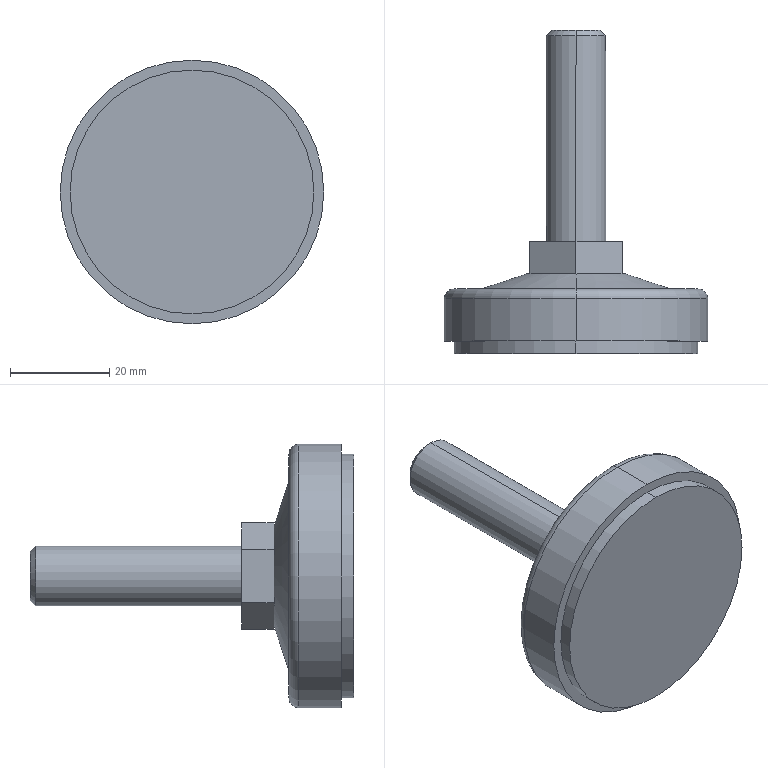Part | STEP file | JAJ-65_adjusters | 1 solid | 35 faces | box 53 x 65 x 53 mm | volume 36497 mm3 | plane 23 | cylinder 6 | cone 4 | torus 2 | commonest cylinder face diameters 12 x2 49 x2 53 x2
STEP:
#1=CARTESIAN_POINT('',(0.000000001,-1.074,6.));
#2=VERTEX_POINT('',#1);
#3=CARTESIAN_POINT('',(-0.000000001,-1.074,-6.));
#4=VERTEX_POINT('',#3);
#5=CARTESIAN_POINT('',(0.,-1.074,0.));
#6=DIRECTION('',(0.,-1.,0.));
#7=DIRECTION('',(0.,0.,-1.));
#8=AXIS2_PLACEMENT_3D('',#5,#6,#7);
#9=CIRCLE('',#8,6.);
#10=EDGE_CURVE('',#2,#4,#9,.T.);
#11=ORIENTED_EDGE('',*,*,#10,.T.);
#12=CARTESIAN_POINT('',(-0.000000005,-42.5,-6.));
#13=VERTEX_POINT('',#12);
#14=CARTESIAN_POINT('',(-0.000000005,-65.,-6.));
#15=DIRECTION('',(0.,-1.,0.));
#16=VECTOR('',#15,1000.);
#17=LINE('',#14,#16);
#18=EDGE_CURVE('',#4,#13,#17,.T.);
#19=ORIENTED_EDGE('',*,*,#18,.T.);
#20=CARTESIAN_POINT('',(-0.000000007,-42.5,6.));
#21=VERTEX_POINT('',#20);
#22=CARTESIAN_POINT('',(0.,-42.5,0.));
#23=DIRECTION('',(0.,1.,0.));
#24=DIRECTION('',(-0.000000001,0.,1.));
#25=AXIS2_PLACEMENT_3D('',#22,#23,#24);
#26=CIRCLE('',#25,6.);
#27=EDGE_CURVE('',#13,#21,#26,.T.);
#28=ORIENTED_EDGE('',*,*,#27,.T.);
#29=CARTESIAN_POINT('',(0.000000005,-65.,6.));
#30=DIRECTION('',(0.,-1.,0.));
#31=VECTOR('',#30,1000.);
#32=LINE('',#29,#31);
#33=EDGE_CURVE('',#2,#21,#32,.T.);
#34=ORIENTED_EDGE('',*,*,#33,.F.);
#35=EDGE_LOOP('',(#11,#19,#28,#34));
#36=FACE_OUTER_BOUND('',#35,.T.);
#37=CARTESIAN_POINT('',(0.,-65.,0.));
#38=DIRECTION('',(0.,-1.,0.));
#39=DIRECTION('',(0.000000001,0.,1.));
#40=AXIS2_PLACEMENT_3D('',#37,#38,#39);
#41=CYLINDRICAL_SURFACE('',#40,6.);
#42=ADVANCED_FACE('',(#36),#41,.T.);
#43=CARTESIAN_POINT('',(0.000000001,0.,4.927));
#44=VERTEX_POINT('',#43);
#45=CARTESIAN_POINT('',(-0.000000001,0.,-4.927));
#46=VERTEX_POINT('',#45);
#47=CARTESIAN_POINT('',(0.,0.,0.));
#48=DIRECTION('',(0.,-1.,0.));
#49=DIRECTION('',(0.,0.,-1.));
#50=AXIS2_PLACEMENT_3D('',#47,#48,#49);
#51=CIRCLE('',#50,4.927);
#52=EDGE_CURVE('',#44,#46,#51,.T.);
#53=ORIENTED_EDGE('',*,*,#52,.T.);
#54=CARTESIAN_POINT('',(-0.000000001,-1.074,-6.));
#55=DIRECTION('',(0.,-0.7071,-0.7071));
#56=VECTOR('',#55,1000.);
#57=LINE('',#54,#56);
#58=EDGE_CURVE('',#46,#4,#57,.T.);
#59=ORIENTED_EDGE('',*,*,#58,.T.);
#60=ORIENTED_EDGE('',*,*,#10,.F.);
#61=CARTESIAN_POINT('',(0.000000001,-1.074,6.));
#62=DIRECTION('',(0.,-0.7071,0.7071));
#63=VECTOR('',#62,1000.);
#64=LINE('',#61,#63);
#65=EDGE_CURVE('',#44,#2,#64,.T.);
#66=ORIENTED_EDGE('',*,*,#65,.F.);
#67=EDGE_LOOP('',(#53,#59,#60,#66));
#68=FACE_OUTER_BOUND('',#67,.T.);
#69=CARTESIAN_POINT('',(0.,-1.074,0.));
#70=DIRECTION('',(0.,-1.,0.));
#71=DIRECTION('',(0.,0.,1.));
#72=AXIS2_PLACEMENT_3D('',#69,#70,#71);
#73=CONICAL_SURFACE('',#72,6.,0.7854);
#74=ADVANCED_FACE('',(#68),#73,.T.);
#75=CARTESIAN_POINT('',(0.,-62.5,24.5));
#76=VERTEX_POINT('',#75);
#77=CARTESIAN_POINT('',(0.,-62.5,-24.5));
#78=VERTEX_POINT('',#77);
#79=CARTESIAN_POINT('',(0.,-62.5,0.));
#80=DIRECTION('',(0.,-1.,0.));
#81=DIRECTION('',(0.,0.,-1.));
#82=AXIS2_PLACEMENT_3D('',#79,#80,#81);
#83=CIRCLE('',#82,24.5);
#84=EDGE_CURVE('',#76,#78,#83,.T.);
#85=ORIENTED_EDGE('',*,*,#84,.T.);
#86=CARTESIAN_POINT('',(0.,-65.,-24.5));
#87=VERTEX_POINT('',#86);
#88=CARTESIAN_POINT('',(0.,-65.,-24.5));
#89=DIRECTION('',(0.,-1.,0.));
#90=VECTOR('',#89,1000.);
#91=LINE('',#88,#90);
#92=EDGE_CURVE('',#78,#87,#91,.T.);
#93=ORIENTED_EDGE('',*,*,#92,.T.);
#94=CARTESIAN_POINT('',(-0.000000029,-65.,24.5));
#95=VERTEX_POINT('',#94);
#96=CARTESIAN_POINT('',(0.,-65.,0.));
#97=DIRECTION('',(0.,-1.,0.));
#98=DIRECTION('',(-0.000000001,0.,1.));
#99=AXIS2_PLACEMENT_3D('',#96,#97,#98);
#100=CIRCLE('',#99,24.5);
#101=EDGE_CURVE('',#95,#87,#100,.T.);
#102=ORIENTED_EDGE('',*,*,#101,.F.);
#103=CARTESIAN_POINT('',(0.,-65.,24.5));
#104=DIRECTION('',(0.,-1.,0.));
#105=VECTOR('',#104,1000.);
#106=LINE('',#103,#105);
#107=EDGE_CURVE('',#76,#95,#106,.T.);
#108=ORIENTED_EDGE('',*,*,#107,.F.);
#109=EDGE_LOOP('',(#85,#93,#102,#108));
#110=FACE_OUTER_BOUND('',#109,.T.);
#111=CARTESIAN_POINT('',(0.,-65.,0.));
#112=DIRECTION('',(0.,-1.,0.));
#113=DIRECTION('',(0.,0.,1.));
#114=AXIS2_PLACEMENT_3D('',#111,#112,#113);
#115=CYLINDRICAL_SURFACE('',#114,24.5);
#116=ADVANCED_FACE('',(#110),#115,.T.);
#117=CARTESIAN_POINT('',(0.,-54.,26.5));
#118=VERTEX_POINT('',#117);
#119=CARTESIAN_POINT('',(0.,-54.,-26.5));
#120=VERTEX_POINT('',#119);
#121=CARTESIAN_POINT('',(0.,-54.,0.));
#122=DIRECTION('',(0.,-1.,0.));
#123=DIRECTION('',(0.,0.,-1.));
#124=AXIS2_PLACEMENT_3D('',#121,#122,#123);
#125=CIRCLE('',#124,26.5);
#126=EDGE_CURVE('',#118,#120,#125,.T.);
#127=ORIENTED_EDGE('',*,*,#126,.T.);
#128=CARTESIAN_POINT('',(0.,-62.5,-26.5));
#129=VERTEX_POINT('',#128);
#130=CARTESIAN_POINT('',(0.,-65.,-26.5));
#131=DIRECTION('',(0.,-1.,0.));
#132=VECTOR('',#131,1000.);
#133=LINE('',#130,#132);
#134=EDGE_CURVE('',#120,#129,#133,.T.);
#135=ORIENTED_EDGE('',*,*,#134,.T.);
#136=CARTESIAN_POINT('',(0.,-62.5,26.5));
#137=VERTEX_POINT('',#136);
#138=CARTESIAN_POINT('',(0.,-62.5,0.));
#139=DIRECTION('',(0.,-1.,0.));
#140=DIRECTION('',(0.,0.,1.));
#141=AXIS2_PLACEMENT_3D('',#138,#139,#140);
#142=CIRCLE('',#141,26.5);
#143=EDGE_CURVE('',#137,#129,#142,.T.);
#144=ORIENTED_EDGE('',*,*,#143,.F.);
#145=CARTESIAN_POINT('',(0.,-65.,26.5));
#146=DIRECTION('',(0.,-1.,0.));
#147=VECTOR('',#146,1000.);
#148=LINE('',#145,#147);
#149=EDGE_CURVE('',#118,#137,#148,.T.);
#150=ORIENTED_EDGE('',*,*,#149,.F.);
#151=EDGE_LOOP('',(#127,#135,#144,#150));
#152=FACE_OUTER_BOUND('',#151,.T.);
#153=CARTESIAN_POINT('',(0.,-65.,0.));
#154=DIRECTION('',(0.,-1.,0.));
#155=DIRECTION('',(0.,0.,1.));
#156=AXIS2_PLACEMENT_3D('',#153,#154,#155);
#157=CYLINDRICAL_SURFACE('',#156,26.5);
#158=ADVANCED_FACE('',(#152),#157,.T.);
#159=CARTESIAN_POINT('',(0.,-52.,24.5));
#160=VERTEX_POINT('',#159);
#161=CARTESIAN_POINT('',(0.,-52.,-24.5));
#162=VERTEX_POINT('',#161);
#163=CARTESIAN_POINT('',(0.,-52.,0.));
#164=DIRECTION('',(0.,-1.,0.));
#165=DIRECTION('',(0.,0.,-1.));
#166=AXIS2_PLACEMENT_3D('',#163,#164,#165);
#167=CIRCLE('',#166,24.5);
#168=EDGE_CURVE('',#160,#162,#167,.T.);
#169=ORIENTED_EDGE('',*,*,#168,.T.);
#170=CARTESIAN_POINT('',(0.,-54.,-24.5));
#171=DIRECTION('',(-1.,0.,0.));
#172=DIRECTION('',(0.,0.,1.));
#173=AXIS2_PLACEMENT_3D('',#170,#171,#172);
#174=CIRCLE('',#173,2.);
#175=EDGE_CURVE('',#162,#120,#174,.T.);
#176=ORIENTED_EDGE('',*,*,#175,.T.);
#177=ORIENTED_EDGE('',*,*,#126,.F.);
#178=CARTESIAN_POINT('',(0.,-54.,24.5));
#179=DIRECTION('',(1.,0.,0.));
#180=DIRECTION('',(0.,0.,-1.));
#181=AXIS2_PLACEMENT_3D('',#178,#179,#180);
#182=CIRCLE('',#181,2.);
#183=EDGE_CURVE('',#160,#118,#182,.T.);
#184=ORIENTED_EDGE('',*,*,#183,.F.);
#185=EDGE_LOOP('',(#169,#176,#177,#184));
#186=FACE_OUTER_BOUND('',#185,.T.);
#187=CARTESIAN_POINT('',(0.,-54.,0.));
#188=DIRECTION('',(0.,-1.,0.));
#189=DIRECTION('',(0.,0.,1.));
#190=AXIS2_PLACEMENT_3D('',#187,#188,#189);
#191=TOROIDAL_SURFACE('',#190,24.5,2.);
#192=ADVANCED_FACE('',(#186),#191,.T.);
#193=CARTESIAN_POINT('',(-1.334,-49.,-9.911));
#194=VERTEX_POINT('',#193);
#195=CARTESIAN_POINT('',(0.,-49.,-10.));
#196=VERTEX_POINT('',#195);
#197=CARTESIAN_POINT('',(0.,-49.,0.));
#198=DIRECTION('',(0.,-1.,0.));
#199=DIRECTION('',(0.,0.,-1.));
#200=AXIS2_PLACEMENT_3D('',#197,#198,#199);
#201=CIRCLE('',#200,10.);
#202=EDGE_CURVE('',#194,#196,#201,.T.);
#203=ORIENTED_EDGE('',*,*,#202,.T.);
#204=CARTESIAN_POINT('',(0.,-52.,-19.));
#205=VERTEX_POINT('',#204);
#206=CARTESIAN_POINT('',(0.,-52.,-19.));
#207=DIRECTION('',(0.,-0.3162,-0.9487));
#208=VECTOR('',#207,1000.);
#209=LINE('',#206,#208);
#210=EDGE_CURVE('',#196,#205,#209,.T.);
#211=ORIENTED_EDGE('',*,*,#210,.T.);
#212=CARTESIAN_POINT('',(0.,-52.,19.));
#213=VERTEX_POINT('',#212);
#214=CARTESIAN_POINT('',(0.,-52.,0.));
#215=DIRECTION('',(0.,-1.,0.));
#216=DIRECTION('',(0.,0.,1.));
#217=AXIS2_PLACEMENT_3D('',#214,#215,#216);
#218=CIRCLE('',#217,19.);
#219=EDGE_CURVE('',#213,#205,#218,.T.);
#220=ORIENTED_EDGE('',*,*,#219,.F.);
#221=CARTESIAN_POINT('',(0.,-49.,10.));
#222=VERTEX_POINT('',#221);
#223=CARTESIAN_POINT('',(0.,-52.,19.));
#224=DIRECTION('',(0.,-0.3162,0.9487));
#225=VECTOR('',#224,1000.);
#226=LINE('',#223,#225);
#227=EDGE_CURVE('',#222,#213,#226,.T.);
#228=ORIENTED_EDGE('',*,*,#227,.F.);
#229=CARTESIAN_POINT('',(-1.334,-49.,9.911));
#230=VERTEX_POINT('',#229);
#231=CARTESIAN_POINT('',(0.,-49.,0.));
#232=DIRECTION('',(0.,-1.,0.));
#233=DIRECTION('',(0.,0.,1.));
#234=AXIS2_PLACEMENT_3D('',#231,#232,#233);
#235=CIRCLE('',#234,10.);
#236=EDGE_CURVE('',#222,#230,#235,.T.);
#237=ORIENTED_EDGE('',*,*,#236,.T.);
#238=CARTESIAN_POINT('',(-7.916,-49.,6.111));
#239=VERTEX_POINT('',#238);
#240=CARTESIAN_POINT('',(0.,-49.,0.));
#241=DIRECTION('',(0.,-1.,0.));
#242=DIRECTION('',(-0.7916,0.,0.6111));
#243=AXIS2_PLACEMENT_3D('',#240,#241,#242);
#244=CIRCLE('',#243,10.);
#245=EDGE_CURVE('',#230,#239,#244,.T.);
#246=ORIENTED_EDGE('',*,*,#245,.T.);
#247=CARTESIAN_POINT('',(-9.25,-49.,3.8));
#248=VERTEX_POINT('',#247);
#249=CARTESIAN_POINT('',(0.,-49.,0.));
#250=DIRECTION('',(0.,-1.,0.));
#251=DIRECTION('',(-0.925,0.,0.38));
#252=AXIS2_PLACEMENT_3D('',#249,#250,#251);
#253=CIRCLE('',#252,10.);
#254=EDGE_CURVE('',#239,#248,#253,.T.);
#255=ORIENTED_EDGE('',*,*,#254,.T.);
#256=CARTESIAN_POINT('',(-9.25,-49.,-3.8));
#257=VERTEX_POINT('',#256);
#258=CARTESIAN_POINT('',(0.,-49.,0.));
#259=DIRECTION('',(0.,-1.,0.));
#260=DIRECTION('',(-0.925,0.,-0.38));
#261=AXIS2_PLACEMENT_3D('',#258,#259,#260);
#262=CIRCLE('',#261,10.);
#263=EDGE_CURVE('',#248,#257,#262,.T.);
#264=ORIENTED_EDGE('',*,*,#263,.T.);
#265=CARTESIAN_POINT('',(-7.916,-49.,-6.111));
#266=VERTEX_POINT('',#265);
#267=CARTESIAN_POINT('',(0.,-49.,0.));
#268=DIRECTION('',(0.,-1.,0.));
#269=DIRECTION('',(-0.7916,0.,-0.6111));
#270=AXIS2_PLACEMENT_3D('',#267,#268,#269);
#271=CIRCLE('',#270,10.);
#272=EDGE_CURVE('',#257,#266,#271,.T.);
#273=ORIENTED_EDGE('',*,*,#272,.T.);
#274=CARTESIAN_POINT('',(0.,-49.,0.));
#275=DIRECTION('',(0.,-1.,0.));
#276=DIRECTION('',(-0.1334,0.,-0.9911));
#277=AXIS2_PLACEMENT_3D('',#274,#275,#276);
#278=CIRCLE('',#277,10.);
#279=EDGE_CURVE('',#266,#194,#278,.T.);
#280=ORIENTED_EDGE('',*,*,#279,.T.);
#281=EDGE_LOOP('',(#203,#211,#220,#228,#237,#246,#255,#264,#273,#280));
#282=FACE_OUTER_BOUND('',#281,.T.);
#283=CARTESIAN_POINT('',(0.,-52.,0.));
#284=DIRECTION('',(0.,-1.,0.));
#285=DIRECTION('',(0.,0.,1.));
#286=AXIS2_PLACEMENT_3D('',#283,#284,#285);
#287=CONICAL_SURFACE('',#286,19.,1.249);
#288=ADVANCED_FACE('',(#282),#287,.T.);
#289=CARTESIAN_POINT('',(-9.25,-49.,3.8));
#290=DIRECTION('',(0.,0.,1.));
#291=VECTOR('',#290,1000.);
#292=LINE('',#289,#291);
#293=EDGE_CURVE('',#257,#248,#292,.T.);
#294=ORIENTED_EDGE('',*,*,#293,.F.);
#295=ORIENTED_EDGE('',*,*,#263,.F.);
#296=EDGE_LOOP('',(#294,#295));
#297=FACE_OUTER_BOUND('',#296,.T.);
#298=CARTESIAN_POINT('',(-10.002,-49.,3.8));
#299=DIRECTION('',(0.,1.,0.));
#300=DIRECTION('',(1.,0.,0.));
#301=AXIS2_PLACEMENT_3D('',#298,#299,#300);
#302=PLANE('',#301);
#303=ADVANCED_FACE('',(#297),#302,.T.);
#304=CARTESIAN_POINT('',(-1.334,-49.,9.911));
#305=DIRECTION('',(0.866,0.,0.5));
#306=VECTOR('',#305,1000.);
#307=LINE('',#304,#306);
#308=EDGE_CURVE('',#239,#230,#307,.T.);
#309=ORIENTED_EDGE('',*,*,#308,.F.);
#310=ORIENTED_EDGE('',*,*,#245,.F.);
#311=EDGE_LOOP('',(#309,#310));
#312=FACE_OUTER_BOUND('',#311,.T.);
#313=CARTESIAN_POINT('',(-7.916,-49.,9.911));
#314=DIRECTION('',(0.,1.,0.));
#315=DIRECTION('',(1.,0.,0.));
#316=AXIS2_PLACEMENT_3D('',#313,#314,#315);
#317=PLANE('',#316);
#318=ADVANCED_FACE('',(#312),#317,.T.);
#319=CARTESIAN_POINT('',(1.334,-49.,9.911));
#320=VERTEX_POINT('',#319);
#321=CARTESIAN_POINT('',(7.916,-49.,6.111));
#322=VERTEX_POINT('',#321);
#323=CARTESIAN_POINT('',(7.916,-49.,6.111));
#324=DIRECTION('',(0.866,0.,-0.5));
#325=VECTOR('',#324,1000.);
#326=LINE('',#323,#325);
#327=EDGE_CURVE('',#320,#322,#326,.T.);
#328=ORIENTED_EDGE('',*,*,#327,.F.);
#329=CARTESIAN_POINT('',(0.,-49.,0.));
#330=DIRECTION('',(0.,-1.,0.));
#331=DIRECTION('',(0.1334,0.,0.9911));
#332=AXIS2_PLACEMENT_3D('',#329,#330,#331);
#333=CIRCLE('',#332,10.);
#334=EDGE_CURVE('',#322,#320,#333,.T.);
#335=ORIENTED_EDGE('',*,*,#334,.F.);
#336=EDGE_LOOP('',(#328,#335));
#337=FACE_OUTER_BOUND('',#336,.T.);
#338=CARTESIAN_POINT('',(1.334,-49.,9.911));
#339=DIRECTION('',(0.,1.,0.));
#340=DIRECTION('',(1.,0.,0.));
#341=AXIS2_PLACEMENT_3D('',#338,#339,#340);
#342=PLANE('',#341);
#343=ADVANCED_FACE('',(#337),#342,.T.);
#344=CARTESIAN_POINT('',(9.25,-49.,-3.8));
#345=VERTEX_POINT('',#344);
#346=CARTESIAN_POINT('',(9.25,-49.,3.8));
#347=VERTEX_POINT('',#346);
#348=CARTESIAN_POINT('',(0.,-49.,0.));
#349=DIRECTION('',(0.,-1.,0.));
#350=DIRECTION('',(0.925,0.,0.38));
#351=AXIS2_PLACEMENT_3D('',#348,#349,#350);
#352=CIRCLE('',#351,10.);
#353=EDGE_CURVE('',#345,#347,#352,.T.);
#354=ORIENTED_EDGE('',*,*,#353,.F.);
#355=CARTESIAN_POINT('',(9.25,-49.,-3.8));
#356=DIRECTION('',(0.,0.,-1.));
#357=VECTOR('',#356,1000.);
#358=LINE('',#355,#357);
#359=EDGE_CURVE('',#347,#345,#358,.T.);
#360=ORIENTED_EDGE('',*,*,#359,.F.);
#361=EDGE_LOOP('',(#354,#360));
#362=FACE_OUTER_BOUND('',#361,.T.);
#363=CARTESIAN_POINT('',(9.25,-49.,3.8));
#364=DIRECTION('',(0.,1.,0.));
#365=DIRECTION('',(1.,0.,0.));
#366=AXIS2_PLACEMENT_3D('',#363,#364,#365);
#367=PLANE('',#366);
#368=ADVANCED_FACE('',(#362),#367,.T.);
#369=CARTESIAN_POINT('',(7.916,-49.,-6.111));
#370=VERTEX_POINT('',#369);
#371=CARTESIAN_POINT('',(1.334,-49.,-9.911));
#372=VERTEX_POINT('',#371);
#373=CARTESIAN_POINT('',(1.334,-49.,-9.911));
#374=DIRECTION('',(-0.866,0.,-0.5));
#375=VECTOR('',#374,1000.);
#376=LINE('',#373,#375);
#377=EDGE_CURVE('',#370,#372,#376,.T.);
#378=ORIENTED_EDGE('',*,*,#377,.F.);
#379=CARTESIAN_POINT('',(0.,-49.,0.));
#380=DIRECTION('',(0.,-1.,0.));
#381=DIRECTION('',(0.7916,0.,-0.6111));
#382=AXIS2_PLACEMENT_3D('',#379,#380,#381);
#383=CIRCLE('',#382,10.);
#384=EDGE_CURVE('',#372,#370,#383,.T.);
#385=ORIENTED_EDGE('',*,*,#384,.F.);
#386=EDGE_LOOP('',(#378,#385));
#387=FACE_OUTER_BOUND('',#386,.T.);
#388=CARTESIAN_POINT('',(1.334,-49.,-6.111));
#389=DIRECTION('',(0.,1.,0.));
#390=DIRECTION('',(1.,0.,0.));
#391=AXIS2_PLACEMENT_3D('',#388,#389,#390);
#392=PLANE('',#391);
#393=ADVANCED_FACE('',(#387),#392,.T.);
#394=CARTESIAN_POINT('',(-7.916,-49.,-6.111));
#395=DIRECTION('',(-0.866,0.,0.5));
#396=VECTOR('',#395,1000.);
#397=LINE('',#394,#396);
#398=EDGE_CURVE('',#194,#266,#397,.T.);
#399=ORIENTED_EDGE('',*,*,#398,.F.);
#400=ORIENTED_EDGE('',*,*,#279,.F.);
#401=EDGE_LOOP('',(#399,#400));
#402=FACE_OUTER_BOUND('',#401,.T.);
#403=CARTESIAN_POINT('',(-7.916,-49.,-6.111));
#404=DIRECTION('',(0.,1.,0.));
#405=DIRECTION('',(1.,0.,0.));
#406=AXIS2_PLACEMENT_3D('',#403,#404,#405);
#407=PLANE('',#406);
#408=ADVANCED_FACE('',(#402),#407,.T.);
#409=ORIENTED_EDGE('',*,*,#168,.F.);
#410=CARTESIAN_POINT('',(0.,-52.,0.));
#411=DIRECTION('',(0.,-1.,0.));
#412=DIRECTION('',(0.,0.,-1.));
#413=AXIS2_PLACEMENT_3D('',#410,#411,#412);
#414=CIRCLE('',#413,24.5);
#415=EDGE_CURVE('',#162,#160,#414,.T.);
#416=ORIENTED_EDGE('',*,*,#415,.F.);
#417=EDGE_LOOP('',(#409,#416));
#418=FACE_OUTER_BOUND('',#417,.T.);
#419=ORIENTED_EDGE('',*,*,#219,.T.);
#420=CARTESIAN_POINT('',(0.,-52.,0.));
#421=DIRECTION('',(0.,-1.,0.));
#422=DIRECTION('',(0.,0.,1.));
#423=AXIS2_PLACEMENT_3D('',#420,#421,#422);
#424=CIRCLE('',#423,19.);
#425=EDGE_CURVE('',#205,#213,#424,.T.);
#426=ORIENTED_EDGE('',*,*,#425,.T.);
#427=EDGE_LOOP('',(#419,#426));
#428=FACE_BOUND('',#427,.T.);
#429=CARTESIAN_POINT('',(-24.955,-52.,24.5));
#430=DIRECTION('',(0.,1.,0.));
#431=DIRECTION('',(1.,0.,0.));
#432=AXIS2_PLACEMENT_3D('',#429,#430,#431);
#433=PLANE('',#432);
#434=ADVANCED_FACE('',(#418,#428),#433,.T.);
#435=ORIENTED_EDGE('',*,*,#143,.T.);
#436=CARTESIAN_POINT('',(0.,-62.5,0.));
#437=DIRECTION('',(0.,-1.,0.));
#438=DIRECTION('',(0.,0.,1.));
#439=AXIS2_PLACEMENT_3D('',#436,#437,#438);
#440=CIRCLE('',#439,26.5);
#441=EDGE_CURVE('',#129,#137,#440,.T.);
#442=ORIENTED_EDGE('',*,*,#441,.T.);
#443=EDGE_LOOP('',(#435,#442));
#444=FACE_OUTER_BOUND('',#443,.T.);
#445=ORIENTED_EDGE('',*,*,#84,.F.);
#446=CARTESIAN_POINT('',(0.,-62.5,0.));
#447=DIRECTION('',(0.,-1.,0.));
#448=DIRECTION('',(0.,0.,-1.));
#449=AXIS2_PLACEMENT_3D('',#446,#447,#448);
#450=CIRCLE('',#449,24.5);
#451=EDGE_CURVE('',#78,#76,#450,.T.);
#452=ORIENTED_EDGE('',*,*,#451,.F.);
#453=EDGE_LOOP('',(#445,#452));
#454=FACE_BOUND('',#453,.T.);
#455=CARTESIAN_POINT('',(-26.992,-62.5,-26.5));
#456=DIRECTION('',(0.,-1.,0.));
#457=DIRECTION('',(1.,0.,0.));
#458=AXIS2_PLACEMENT_3D('',#455,#456,#457);
#459=PLANE('',#458);
#460=ADVANCED_FACE('',(#444,#454),#459,.T.);
#461=ORIENTED_EDGE('',*,*,#101,.T.);
#462=CARTESIAN_POINT('',(0.,-65.,0.));
#463=DIRECTION('',(0.,-1.,0.));
#464=DIRECTION('',(-0.000000001,0.,1.));
#465=AXIS2_PLACEMENT_3D('',#462,#463,#464);
#466=CIRCLE('',#465,24.5);
#467=EDGE_CURVE('',#87,#95,#466,.T.);
#468=ORIENTED_EDGE('',*,*,#467,.T.);
#469=EDGE_LOOP('',(#461,#468));
#470=FACE_OUTER_BOUND('',#469,.T.);
#471=CARTESIAN_POINT('',(-24.955,-65.,-24.5));
#472=DIRECTION('',(0.,-1.,0.));
#473=DIRECTION('',(1.,0.,0.));
#474=AXIS2_PLACEMENT_3D('',#471,#472,#473);
#475=PLANE('',#474);
#476=ADVANCED_FACE('',(#470),#475,.T.);
#477=CARTESIAN_POINT('',(9.25,-49.,5.34));
#478=VERTEX_POINT('',#477);
#479=CARTESIAN_POINT('',(9.25,-49.,5.34));
#480=DIRECTION('',(0.866,0.,-0.5));
#481=VECTOR('',#480,1000.);
#482=LINE('',#479,#481);
#483=EDGE_CURVE('',#322,#478,#482,.T.);
#484=ORIENTED_EDGE('',*,*,#483,.F.);
#485=CARTESIAN_POINT('',(0.,-49.,0.));
#486=DIRECTION('',(0.,-1.,0.));
#487=DIRECTION('',(0.7916,0.,0.6111));
#488=AXIS2_PLACEMENT_3D('',#485,#486,#487);
#489=CIRCLE('',#488,10.);
#490=EDGE_CURVE('',#347,#322,#489,.T.);
#491=ORIENTED_EDGE('',*,*,#490,.F.);
#492=CARTESIAN_POINT('',(9.25,-49.,3.8));
#493=DIRECTION('',(0.,0.,-1.));
#494=VECTOR('',#493,1000.);
#495=LINE('',#492,#494);
#496=EDGE_CURVE('',#478,#347,#495,.T.);
#497=ORIENTED_EDGE('',*,*,#496,.F.);
#498=EDGE_LOOP('',(#484,#491,#497));
#499=FACE_OUTER_BOUND('',#498,.T.);
#500=CARTESIAN_POINT('',(7.916,-49.,3.8));
#501=DIRECTION('',(0.,-1.,0.));
#502=DIRECTION('',(1.,0.,0.));
#503=AXIS2_PLACEMENT_3D('',#500,#501,#502);
#504=PLANE('',#503);
#505=ADVANCED_FACE('',(#499),#504,.T.);
#506=CARTESIAN_POINT('',(9.25,-49.,-5.34));
#507=VERTEX_POINT('',#506);
#508=CARTESIAN_POINT('',(9.25,-49.,-5.34));
#509=DIRECTION('',(0.,0.,-1.));
#510=VECTOR('',#509,1000.);
#511=LINE('',#508,#510);
#512=EDGE_CURVE('',#345,#507,#511,.T.);
#513=ORIENTED_EDGE('',*,*,#512,.F.);
#514=CARTESIAN_POINT('',(0.,-49.,0.));
#515=DIRECTION('',(0.,-1.,0.));
#516=DIRECTION('',(0.925,0.,-0.38));
#517=AXIS2_PLACEMENT_3D('',#514,#515,#516);
#518=CIRCLE('',#517,10.);
#519=EDGE_CURVE('',#370,#345,#518,.T.);
#520=ORIENTED_EDGE('',*,*,#519,.F.);
#521=CARTESIAN_POINT('',(7.916,-49.,-6.111));
#522=DIRECTION('',(-0.866,0.,-0.5));
#523=VECTOR('',#522,1000.);
#524=LINE('',#521,#523);
#525=EDGE_CURVE('',#507,#370,#524,.T.);
#526=ORIENTED_EDGE('',*,*,#525,.F.);
#527=EDGE_LOOP('',(#513,#520,#526));
#528=FACE_OUTER_BOUND('',#527,.T.);
#529=CARTESIAN_POINT('',(7.916,-49.,-6.111));
#530=DIRECTION('',(0.,-1.,0.));
#531=DIRECTION('',(1.,0.,0.));
#532=AXIS2_PLACEMENT_3D('',#529,#530,#531);
#533=PLANE('',#532);
#534=ADVANCED_FACE('',(#528),#533,.T.);
#535=CARTESIAN_POINT('',(0.,-49.,-10.681));
#536=VERTEX_POINT('',#535);
#537=CARTESIAN_POINT('',(0.,-49.,-10.681));
#538=DIRECTION('',(-0.866,0.,-0.5));
#539=VECTOR('',#538,1000.);
#540=LINE('',#537,#539);
#541=EDGE_CURVE('',#372,#536,#540,.T.);
#542=ORIENTED_EDGE('',*,*,#541,.F.);
#543=CARTESIAN_POINT('',(0.,-49.,0.));
#544=DIRECTION('',(0.,-1.,0.));
#545=DIRECTION('',(0.,0.,-1.));
#546=AXIS2_PLACEMENT_3D('',#543,#544,#545);
#547=CIRCLE('',#546,10.);
#548=EDGE_CURVE('',#196,#372,#547,.T.);
#549=ORIENTED_EDGE('',*,*,#548,.F.);
#550=ORIENTED_EDGE('',*,*,#202,.F.);
#551=CARTESIAN_POINT('',(-1.334,-49.,-9.911));
#552=DIRECTION('',(-0.866,0.,0.5));
#553=VECTOR('',#552,1000.);
#554=LINE('',#551,#553);
#555=EDGE_CURVE('',#536,#194,#554,.T.);
#556=ORIENTED_EDGE('',*,*,#555,.F.);
#557=EDGE_LOOP('',(#542,#549,#550,#556));
#558=FACE_OUTER_BOUND('',#557,.T.);
#559=CARTESIAN_POINT('',(-1.334,-49.,-10.681));
#560=DIRECTION('',(0.,-1.,0.));
#561=DIRECTION('',(1.,0.,0.));
#562=AXIS2_PLACEMENT_3D('',#559,#560,#561);
#563=PLANE('',#562);
#564=ADVANCED_FACE('',(#558),#563,.T.);
#565=CARTESIAN_POINT('',(-9.25,-49.,-5.34));
#566=VERTEX_POINT('',#565);
#567=CARTESIAN_POINT('',(-9.25,-49.,-5.34));
#568=DIRECTION('',(-0.866,0.,0.5));
#569=VECTOR('',#568,1000.);
#570=LINE('',#567,#569);
#571=EDGE_CURVE('',#266,#566,#570,.T.);
#572=ORIENTED_EDGE('',*,*,#571,.F.);
#573=ORIENTED_EDGE('',*,*,#272,.F.);
#574=CARTESIAN_POINT('',(-9.25,-49.,-3.8));
#575=DIRECTION('',(0.,0.,1.));
#576=VECTOR('',#575,1000.);
#577=LINE('',#574,#576);
#578=EDGE_CURVE('',#566,#257,#577,.T.);
#579=ORIENTED_EDGE('',*,*,#578,.F.);
#580=EDGE_LOOP('',(#572,#573,#579));
#581=FACE_OUTER_BOUND('',#580,.T.);
#582=CARTESIAN_POINT('',(-9.25,-49.,-6.111));
#583=DIRECTION('',(0.,-1.,0.));
#584=DIRECTION('',(1.,0.,0.));
#585=AXIS2_PLACEMENT_3D('',#582,#583,#584);
#586=PLANE('',#585);
#587=ADVANCED_FACE('',(#581),#586,.T.);
#588=CARTESIAN_POINT('',(-9.25,-49.,5.34));
#589=VERTEX_POINT('',#588);
#590=CARTESIAN_POINT('',(-9.25,-49.,5.34));
#591=DIRECTION('',(0.,0.,1.));
#592=VECTOR('',#591,1000.);
#593=LINE('',#590,#592);
#594=EDGE_CURVE('',#248,#589,#593,.T.);
#595=ORIENTED_EDGE('',*,*,#594,.F.);
#596=ORIENTED_EDGE('',*,*,#254,.F.);
#597=CARTESIAN_POINT('',(-7.916,-49.,6.111));
#598=DIRECTION('',(0.866,0.,0.5));
#599=VECTOR('',#598,1000.);
#600=LINE('',#597,#599);
#601=EDGE_CURVE('',#589,#239,#600,.T.);
#602=ORIENTED_EDGE('',*,*,#601,.F.);
#603=EDGE_LOOP('',(#595,#596,#602));
#604=FACE_OUTER_BOUND('',#603,.T.);
#605=CARTESIAN_POINT('',(-9.25,-49.,3.8));
#606=DIRECTION('',(0.,-1.,0.));
#607=DIRECTION('',(1.,0.,0.));
#608=AXIS2_PLACEMENT_3D('',#605,#606,#607);
#609=PLANE('',#608);
#610=ADVANCED_FACE('',(#604),#609,.T.);
#611=ORIENTED_EDGE('',*,*,#578,.T.);
#612=ORIENTED_EDGE('',*,*,#293,.T.);
#613=ORIENTED_EDGE('',*,*,#594,.T.);
#614=CARTESIAN_POINT('',(-9.25,-42.5,5.34));
#615=VERTEX_POINT('',#614);
#616=CARTESIAN_POINT('',(-9.25,-49.,5.34));
#617=DIRECTION('',(0.,-1.,0.));
#618=VECTOR('',#617,1000.);
#619=LINE('',#616,#618);
#620=EDGE_CURVE('',#615,#589,#619,.T.);
#621=ORIENTED_EDGE('',*,*,#620,.F.);
#622=CARTESIAN_POINT('',(-9.25,-42.5,-5.34));
#623=VERTEX_POINT('',#622);
#624=CARTESIAN_POINT('',(-9.25,-42.5,5.34));
#625=DIRECTION('',(0.,0.,1.));
#626=VECTOR('',#625,1000.);
#627=LINE('',#624,#626);
#628=EDGE_CURVE('',#623,#615,#627,.T.);
#629=ORIENTED_EDGE('',*,*,#628,.F.);
#630=CARTESIAN_POINT('',(-9.25,-42.5,-5.34));
#631=DIRECTION('',(0.,-1.,0.));
#632=VECTOR('',#631,1000.);
#633=LINE('',#630,#632);
#634=EDGE_CURVE('',#623,#566,#633,.T.);
#635=ORIENTED_EDGE('',*,*,#634,.T.);
#636=EDGE_LOOP('',(#611,#612,#613,#621,#629,#635));
#637=FACE_OUTER_BOUND('',#636,.T.);
#638=CARTESIAN_POINT('',(-9.25,-49.,5.34));
#639=DIRECTION('',(-1.,0.,0.));
#640=DIRECTION('',(0.,1.,0.));
#641=AXIS2_PLACEMENT_3D('',#638,#639,#640);
#642=PLANE('',#641);
#643=ADVANCED_FACE('',(#637),#642,.T.);
#644=ORIENTED_EDGE('',*,*,#601,.T.);
#645=ORIENTED_EDGE('',*,*,#308,.T.);
#646=CARTESIAN_POINT('',(0.,-49.,10.681));
#647=VERTEX_POINT('',#646);
#648=CARTESIAN_POINT('',(-1.334,-49.,9.911));
#649=DIRECTION('',(0.866,0.,0.5));
#650=VECTOR('',#649,1000.);
#651=LINE('',#648,#650);
#652=EDGE_CURVE('',#230,#647,#651,.T.);
#653=ORIENTED_EDGE('',*,*,#652,.T.);
#654=CARTESIAN_POINT('',(0.,-42.5,10.681));
#655=VERTEX_POINT('',#654);
#656=CARTESIAN_POINT('',(0.,-49.,10.681));
#657=DIRECTION('',(0.,-1.,0.));
#658=VECTOR('',#657,1000.);
#659=LINE('',#656,#658);
#660=EDGE_CURVE('',#655,#647,#659,.T.);
#661=ORIENTED_EDGE('',*,*,#660,.F.);
#662=CARTESIAN_POINT('',(0.,-42.5,10.681));
#663=DIRECTION('',(0.866,0.,0.5));
#664=VECTOR('',#663,1000.);
#665=LINE('',#662,#664);
#666=EDGE_CURVE('',#615,#655,#665,.T.);
#667=ORIENTED_EDGE('',*,*,#666,.F.);
#668=ORIENTED_EDGE('',*,*,#620,.T.);
#669=EDGE_LOOP('',(#644,#645,#653,#661,#667,#668));
#670=FACE_OUTER_BOUND('',#669,.T.);
#671=CARTESIAN_POINT('',(0.,-49.,10.681));
#672=DIRECTION('',(-0.5,0.,0.866));
#673=DIRECTION('',(0.,1.,0.));
#674=AXIS2_PLACEMENT_3D('',#671,#672,#673);
#675=PLANE('',#674);
#676=ADVANCED_FACE('',(#670),#675,.T.);
#677=CARTESIAN_POINT('',(0.,-49.,10.681));
#678=DIRECTION('',(0.866,0.,-0.5));
#679=VECTOR('',#678,1000.);
#680=LINE('',#677,#679);
#681=EDGE_CURVE('',#647,#320,#680,.T.);
#682=ORIENTED_EDGE('',*,*,#681,.T.);
#683=ORIENTED_EDGE('',*,*,#327,.T.);
#684=ORIENTED_EDGE('',*,*,#483,.T.);
#685=CARTESIAN_POINT('',(9.25,-42.5,5.34));
#686=VERTEX_POINT('',#685);
#687=CARTESIAN_POINT('',(9.25,-49.,5.34));
#688=DIRECTION('',(0.,-1.,0.));
#689=VECTOR('',#688,1000.);
#690=LINE('',#687,#689);
#691=EDGE_CURVE('',#686,#478,#690,.T.);
#692=ORIENTED_EDGE('',*,*,#691,.F.);
#693=CARTESIAN_POINT('',(9.25,-42.5,5.34));
#694=DIRECTION('',(0.866,0.,-0.5));
#695=VECTOR('',#694,1000.);
#696=LINE('',#693,#695);
#697=EDGE_CURVE('',#655,#686,#696,.T.);
#698=ORIENTED_EDGE('',*,*,#697,.F.);
#699=ORIENTED_EDGE('',*,*,#660,.T.);
#700=EDGE_LOOP('',(#682,#683,#684,#692,#698,#699));
#701=FACE_OUTER_BOUND('',#700,.T.);
#702=CARTESIAN_POINT('',(9.25,-49.,5.34));
#703=DIRECTION('',(0.5,0.,0.866));
#704=DIRECTION('',(0.,1.,0.));
#705=AXIS2_PLACEMENT_3D('',#702,#703,#704);
#706=PLANE('',#705);
#707=ADVANCED_FACE('',(#701),#706,.T.);
#708=ORIENTED_EDGE('',*,*,#496,.T.);
#709=ORIENTED_EDGE('',*,*,#359,.T.);
#710=ORIENTED_EDGE('',*,*,#512,.T.);
#711=CARTESIAN_POINT('',(9.25,-42.5,-5.34));
#712=VERTEX_POINT('',#711);
#713=CARTESIAN_POINT('',(9.25,-49.,-5.34));
#714=DIRECTION('',(0.,-1.,0.));
#715=VECTOR('',#714,1000.);
#716=LINE('',#713,#715);
#717=EDGE_CURVE('',#712,#507,#716,.T.);
#718=ORIENTED_EDGE('',*,*,#717,.F.);
#719=CARTESIAN_POINT('',(9.25,-42.5,-5.34));
#720=DIRECTION('',(0.,0.,-1.));
#721=VECTOR('',#720,1000.);
#722=LINE('',#719,#721);
#723=EDGE_CURVE('',#686,#712,#722,.T.);
#724=ORIENTED_EDGE('',*,*,#723,.F.);
#725=ORIENTED_EDGE('',*,*,#691,.T.);
#726=EDGE_LOOP('',(#708,#709,#710,#718,#724,#725));
#727=FACE_OUTER_BOUND('',#726,.T.);
#728=CARTESIAN_POINT('',(9.25,-49.,-5.34));
#729=DIRECTION('',(1.,0.,0.));
#730=DIRECTION('',(0.,1.,0.));
#731=AXIS2_PLACEMENT_3D('',#728,#729,#730);
#732=PLANE('',#731);
#733=ADVANCED_FACE('',(#727),#732,.T.);
#734=ORIENTED_EDGE('',*,*,#525,.T.);
#735=ORIENTED_EDGE('',*,*,#377,.T.);
#736=ORIENTED_EDGE('',*,*,#541,.T.);
#737=CARTESIAN_POINT('',(0.,-42.5,-10.681));
#738=VERTEX_POINT('',#737);
#739=CARTESIAN_POINT('',(0.,-49.,-10.681));
#740=DIRECTION('',(0.,-1.,0.));
#741=VECTOR('',#740,1000.);
#742=LINE('',#739,#741);
#743=EDGE_CURVE('',#738,#536,#742,.T.);
#744=ORIENTED_EDGE('',*,*,#743,.F.);
#745=CARTESIAN_POINT('',(0.,-42.5,-10.681));
#746=DIRECTION('',(-0.866,0.,-0.5));
#747=VECTOR('',#746,1000.);
#748=LINE('',#745,#747);
#749=EDGE_CURVE('',#712,#738,#748,.T.);
#750=ORIENTED_EDGE('',*,*,#749,.F.);
#751=ORIENTED_EDGE('',*,*,#717,.T.);
#752=EDGE_LOOP('',(#734,#735,#736,#744,#750,#751));
#753=FACE_OUTER_BOUND('',#752,.T.);
#754=CARTESIAN_POINT('',(0.,-49.,-10.681));
#755=DIRECTION('',(0.5,0.,-0.866));
#756=DIRECTION('',(0.,1.,0.));
#757=AXIS2_PLACEMENT_3D('',#754,#755,#756);
#758=PLANE('',#757);
#759=ADVANCED_FACE('',(#753),#758,.T.);
#760=ORIENTED_EDGE('',*,*,#555,.T.);
#761=ORIENTED_EDGE('',*,*,#398,.T.);
#762=ORIENTED_EDGE('',*,*,#571,.T.);
#763=ORIENTED_EDGE('',*,*,#634,.F.);
#764=CARTESIAN_POINT('',(-9.25,-42.5,-5.34));
#765=DIRECTION('',(-0.866,0.,0.5));
#766=VECTOR('',#765,1000.);
#767=LINE('',#764,#766);
#768=EDGE_CURVE('',#738,#623,#767,.T.);
#769=ORIENTED_EDGE('',*,*,#768,.F.);
#770=ORIENTED_EDGE('',*,*,#743,.T.);
#771=EDGE_LOOP('',(#760,#761,#762,#763,#769,#770));
#772=FACE_OUTER_BOUND('',#771,.T.);
#773=CARTESIAN_POINT('',(-9.25,-49.,-5.34));
#774=DIRECTION('',(-0.5,0.,-0.866));
#775=DIRECTION('',(0.,1.,0.));
#776=AXIS2_PLACEMENT_3D('',#773,#774,#775);
#777=PLANE('',#776);
#778=ADVANCED_FACE('',(#772),#777,.T.);
#779=ORIENTED_EDGE('',*,*,#628,.T.);
#780=ORIENTED_EDGE('',*,*,#666,.T.);
#781=ORIENTED_EDGE('',*,*,#697,.T.);
#782=ORIENTED_EDGE('',*,*,#723,.T.);
#783=ORIENTED_EDGE('',*,*,#749,.T.);
#784=ORIENTED_EDGE('',*,*,#768,.T.);
#785=EDGE_LOOP('',(#779,#780,#781,#782,#783,#784));
#786=FACE_OUTER_BOUND('',#785,.T.);
#787=CARTESIAN_POINT('',(0.,-42.5,0.));
#788=DIRECTION('',(0.,1.,0.));
#789=DIRECTION('',(-0.000000001,0.,1.));
#790=AXIS2_PLACEMENT_3D('',#787,#788,#789);
#791=CIRCLE('',#790,6.);
#792=EDGE_CURVE('',#21,#13,#791,.T.);
#793=ORIENTED_EDGE('',*,*,#792,.F.);
#794=ORIENTED_EDGE('',*,*,#27,.F.);
#795=EDGE_LOOP('',(#793,#794));
#796=FACE_BOUND('',#795,.T.);
#797=CARTESIAN_POINT('',(-9.25,-42.5,-10.681));
#798=DIRECTION('',(0.,1.,0.));
#799=DIRECTION('',(0.,0.,1.));
#800=AXIS2_PLACEMENT_3D('',#797,#798,#799);
#801=PLANE('',#800);
#802=ADVANCED_FACE('',(#786,#796),#801,.T.);
#803=ORIENTED_EDGE('',*,*,#652,.F.);
#804=ORIENTED_EDGE('',*,*,#236,.F.);
#805=CARTESIAN_POINT('',(0.,-49.,0.));
#806=DIRECTION('',(0.,-1.,0.));
#807=DIRECTION('',(0.,0.,1.));
#808=AXIS2_PLACEMENT_3D('',#805,#806,#807);
#809=CIRCLE('',#808,10.);
#810=EDGE_CURVE('',#320,#222,#809,.T.);
#811=ORIENTED_EDGE('',*,*,#810,.F.);
#812=ORIENTED_EDGE('',*,*,#681,.F.);
#813=EDGE_LOOP('',(#803,#804,#811,#812));
#814=FACE_OUTER_BOUND('',#813,.T.);
#815=CARTESIAN_POINT('',(-1.334,-49.,9.911));
#816=DIRECTION('',(0.,-1.,0.));
#817=DIRECTION('',(1.,0.,0.));
#818=AXIS2_PLACEMENT_3D('',#815,#816,#817);
#819=PLANE('',#818);
#820=ADVANCED_FACE('',(#814),#819,.T.);
#821=ORIENTED_EDGE('',*,*,#52,.F.);
#822=CARTESIAN_POINT('',(0.,0.,0.));
#823=DIRECTION('',(0.,-1.,0.));
#824=DIRECTION('',(0.,0.,-1.));
#825=AXIS2_PLACEMENT_3D('',#822,#823,#824);
#826=CIRCLE('',#825,4.927);
#827=EDGE_CURVE('',#46,#44,#826,.T.);
#828=ORIENTED_EDGE('',*,*,#827,.F.);
#829=EDGE_LOOP('',(#821,#828));
#830=FACE_OUTER_BOUND('',#829,.T.);
#831=CARTESIAN_POINT('',(-4.927,0.,4.927));
#832=DIRECTION('',(0.,1.,0.));
#833=DIRECTION('',(1.,0.,0.));
#834=AXIS2_PLACEMENT_3D('',#831,#832,#833);
#835=PLANE('',#834);
#836=ADVANCED_FACE('',(#830),#835,.T.);
#837=ORIENTED_EDGE('',*,*,#210,.F.);
#838=ORIENTED_EDGE('',*,*,#548,.T.);
#839=ORIENTED_EDGE('',*,*,#384,.T.);
#840=ORIENTED_EDGE('',*,*,#519,.T.);
#841=ORIENTED_EDGE('',*,*,#353,.T.);
#842=ORIENTED_EDGE('',*,*,#490,.T.);
#843=ORIENTED_EDGE('',*,*,#334,.T.);
#844=ORIENTED_EDGE('',*,*,#810,.T.);
#845=ORIENTED_EDGE('',*,*,#227,.T.);
#846=ORIENTED_EDGE('',*,*,#425,.F.);
#847=EDGE_LOOP('',(#837,#838,#839,#840,#841,#842,#843,#844,#845,#846));
#848=FACE_OUTER_BOUND('',#847,.T.);
#849=CARTESIAN_POINT('',(0.,-52.,0.));
#850=DIRECTION('',(0.,-1.,0.));
#851=DIRECTION('',(0.,0.,1.));
#852=AXIS2_PLACEMENT_3D('',#849,#850,#851);
#853=CONICAL_SURFACE('',#852,19.,1.249);
#854=ADVANCED_FACE('',(#848),#853,.T.);
#855=ORIENTED_EDGE('',*,*,#175,.F.);
#856=ORIENTED_EDGE('',*,*,#415,.T.);
#857=ORIENTED_EDGE('',*,*,#183,.T.);
#858=CARTESIAN_POINT('',(0.,-54.,0.));
#859=DIRECTION('',(0.,-1.,0.));
#860=DIRECTION('',(0.,0.,-1.));
#861=AXIS2_PLACEMENT_3D('',#858,#859,#860);
#862=CIRCLE('',#861,26.5);
#863=EDGE_CURVE('',#120,#118,#862,.T.);
#864=ORIENTED_EDGE('',*,*,#863,.F.);
#865=EDGE_LOOP('',(#855,#856,#857,#864));
#866=FACE_OUTER_BOUND('',#865,.T.);
#867=CARTESIAN_POINT('',(0.,-54.,0.));
#868=DIRECTION('',(0.,-1.,0.));
#869=DIRECTION('',(0.,0.,1.));
#870=AXIS2_PLACEMENT_3D('',#867,#868,#869);
#871=TOROIDAL_SURFACE('',#870,24.5,2.);
#872=ADVANCED_FACE('',(#866),#871,.T.);
#873=ORIENTED_EDGE('',*,*,#134,.F.);
#874=ORIENTED_EDGE('',*,*,#863,.T.);
#875=ORIENTED_EDGE('',*,*,#149,.T.);
#876=ORIENTED_EDGE('',*,*,#441,.F.);
#877=EDGE_LOOP('',(#873,#874,#875,#876));
#878=FACE_OUTER_BOUND('',#877,.T.);
#879=CARTESIAN_POINT('',(0.,-65.,0.));
#880=DIRECTION('',(0.,-1.,0.));
#881=DIRECTION('',(0.,0.,1.));
#882=AXIS2_PLACEMENT_3D('',#879,#880,#881);
#883=CYLINDRICAL_SURFACE('',#882,26.5);
#884=ADVANCED_FACE('',(#878),#883,.T.);
#885=ORIENTED_EDGE('',*,*,#92,.F.);
#886=ORIENTED_EDGE('',*,*,#451,.T.);
#887=ORIENTED_EDGE('',*,*,#107,.T.);
#888=ORIENTED_EDGE('',*,*,#467,.F.);
#889=EDGE_LOOP('',(#885,#886,#887,#888));
#890=FACE_OUTER_BOUND('',#889,.T.);
#891=CARTESIAN_POINT('',(0.,-65.,0.));
#892=DIRECTION('',(0.,-1.,0.));
#893=DIRECTION('',(0.,0.,1.));
#894=AXIS2_PLACEMENT_3D('',#891,#892,#893);
#895=CYLINDRICAL_SURFACE('',#894,24.5);
#896=ADVANCED_FACE('',(#890),#895,.T.);
#897=ORIENTED_EDGE('',*,*,#58,.F.);
#898=ORIENTED_EDGE('',*,*,#827,.T.);
#899=ORIENTED_EDGE('',*,*,#65,.T.);
#900=CARTESIAN_POINT('',(0.,-1.074,0.));
#901=DIRECTION('',(0.,-1.,0.));
#902=DIRECTION('',(0.,0.,-1.));
#903=AXIS2_PLACEMENT_3D('',#900,#901,#902);
#904=CIRCLE('',#903,6.);
#905=EDGE_CURVE('',#4,#2,#904,.T.);
#906=ORIENTED_EDGE('',*,*,#905,.F.);
#907=EDGE_LOOP('',(#897,#898,#899,#906));
#908=FACE_OUTER_BOUND('',#907,.T.);
#909=CARTESIAN_POINT('',(0.,-1.074,0.));
#910=DIRECTION('',(0.,-1.,0.));
#911=DIRECTION('',(0.,0.,1.));
#912=AXIS2_PLACEMENT_3D('',#909,#910,#911);
#913=CONICAL_SURFACE('',#912,6.,0.7854);
#914=ADVANCED_FACE('',(#908),#913,.T.);
#915=ORIENTED_EDGE('',*,*,#18,.F.);
#916=ORIENTED_EDGE('',*,*,#905,.T.);
#917=ORIENTED_EDGE('',*,*,#33,.T.);
#918=ORIENTED_EDGE('',*,*,#792,.T.);
#919=EDGE_LOOP('',(#915,#916,#917,#918));
#920=FACE_OUTER_BOUND('',#919,.T.);
#921=CARTESIAN_POINT('',(0.,-65.,0.));
#922=DIRECTION('',(0.,-1.,0.));
#923=DIRECTION('',(0.000000001,0.,1.));
#924=AXIS2_PLACEMENT_3D('',#921,#922,#923);
#925=CYLINDRICAL_SURFACE('',#924,6.);
#926=ADVANCED_FACE('',(#920),#925,.T.);
#927=CLOSED_SHELL('',(#42,#74,#116,#158,#192,#288,#303,#318,#343,#368,#393,#408,#434,#460,#476,#505,#534,#564,#587,#610,#643,#676,#707,#733,#759,#778,#802,#820,#836,#854,#872,#884,#896,#914,#926));
#928=MANIFOLD_SOLID_BREP('',#927);
#929=CARTESIAN_POINT('',(0.,0.,0.));
#930=DIRECTION('',(0.,0.,1.));
#931=DIRECTION('',(1.,0.,0.));
#932=AXIS2_PLACEMENT_3D('',#929,#930,#931);
#933=(LENGTH_UNIT()NAMED_UNIT(*)SI_UNIT(.MILLI.,.METRE.));
#934=UNCERTAINTY_MEASURE_WITH_UNIT(LENGTH_MEASURE(0.00001),#933,'','');
#935=(NAMED_UNIT(*)PLANE_ANGLE_UNIT()SI_UNIT($,.RADIAN.));
#936=(NAMED_UNIT(*)SI_UNIT($,.STERADIAN.)SOLID_ANGLE_UNIT());
#937=(GEOMETRIC_REPRESENTATION_CONTEXT(3)GLOBAL_UNCERTAINTY_ASSIGNED_CONTEXT((#934))GLOBAL_UNIT_ASSIGNED_CONTEXT((#933,#935,#936))REPRESENTATION_CONTEXT('',''));
#938=ADVANCED_BREP_SHAPE_REPRESENTATION('',(#928,#932),#937);